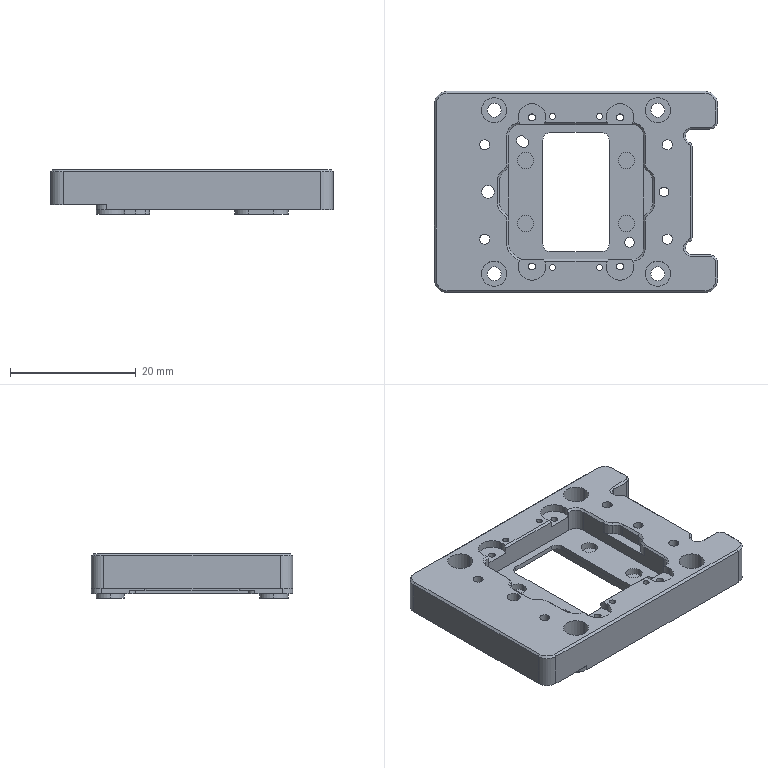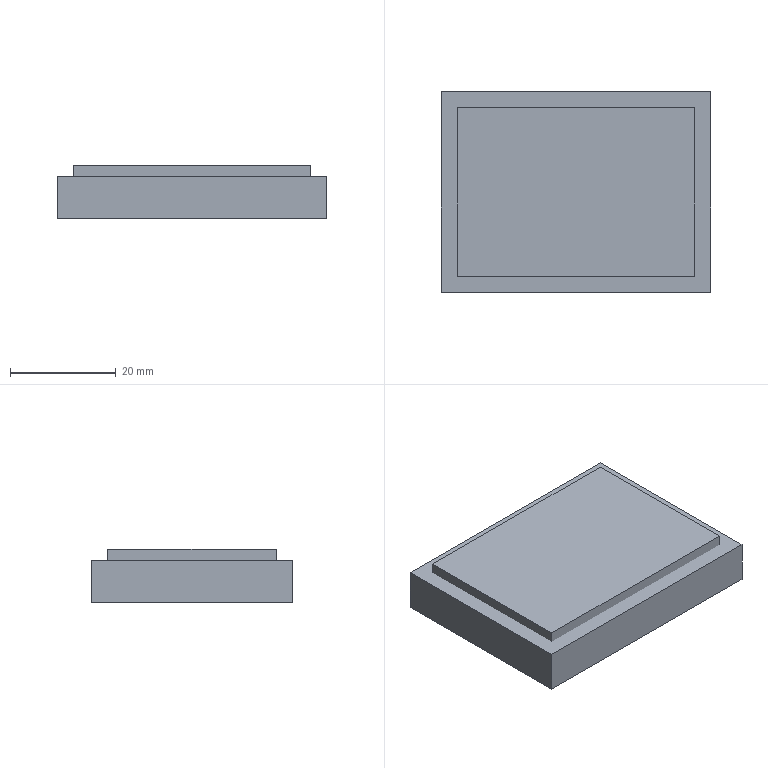CAM job | NX | 3-axis milling, drilling | part box 45 x 32 x 7.05 mm | stock box 51 x 38 x 10.05 mm
Tools:
number,name,description,diameter,corner_radius,flute_length,length,flutes
3,D63,Milling Tool-5 Parameters,63.0,0.0,50.0,75.0,2
1,D6A45,Milling Tool-5 Parameters,6.0,0.0,50.0,75.0,2
11,1.6ZT,Drilling Tool,1.6,0.0,35.0,50.0,2
20,1.55ZT,Drilling Tool,1.55,0.0,35.0,50.0,2
12,2.2ZT,Drilling Tool,2.2,0.0,35.0,50.0,2
13,1.1ZT,Drilling Tool,1.1,0.0,35.0,50.0,2
8,0.95ZT,Drilling Tool,0.95,0.0,35.0,50.0,2
9,2.05ZT,Drilling Tool,2.05,0.0,35.0,50.0,2
6,D6,Milling Tool-5 Parameters,6.0,0.0,50.0,75.0,2
17,D3,Milling Tool-5 Parameters,3.0,0.0,50.0,75.0,2
19,D1.5,Milling Tool-5 Parameters,1.5,0.0,50.0,75.0,2
21,D1,Milling Tool-5 Parameters,1.0,0.0,50.0,75.0,2
18,1.17ZT,Drilling Tool,1.17,0.0,35.0,50.0,2
15,D2,Milling Tool-5 Parameters,2.0,0.0,50.0,75.0,2
15,R0.75,Milling Tool-5 Parameters,0.05,0.025,50.0,75.0,2
Operations:
program,operation,operation_type,tool,method,geometry_group,spindle_rpm,surface_speed,feed_per_tooth,feed_cut,feed_plunge,cut_length_mm,path_length_mm,cut_time_min,machine_time_min
1,FLOOR_WALL,VolumeBased25DMillingOperation,D63,METHOD,A,6500.0,1286.0,0.0962,1250.0,100.0,126.0,180.0,0.1008,0.1062
1,DRILLING,Operation,D6A45,METHOD,A,5000.0,94.0,0.025,250.0,0.0,86.4,459.336,0.3456,0.3829
1,DRILLING_COPY,Operation,1.6ZT,METHOD,A,2000.0,10.0,0.025,100.0,0.0,43.323,215.394,0.4332,0.4504
1,DRILLING_COPY_COPY_1,Operation,1.55ZT,METHOD,A,2000.0,10.0,0.025,100.0,0.0,10.816,81.631,0.1082,0.1152
1,DRILLING_COPY_COPY,Operation,2.2ZT,METHOD,A,1447.0,10.0,0.0346,100.0,0.0,48.844,255.924,0.4884,0.5091
1,DRILLING_COPY_COPY_1_COPY,Operation,1.1ZT,METHOD,A,2000.0,10.0,0.025,100.0,0.0,46.122,213.768,0.4612,0.478
1,DRILLING_COPY_COPY_1_COPY_COPY,Operation,0.95ZT,METHOD,A,2000.0,10.0,0.025,100.0,0.0,37.542,184.425,0.3754,0.3901
1,DRILLING_COPY_COPY_COPY,Operation,2.05ZT,METHOD,A,1447.0,10.0,0.0346,100.0,0.0,10.966,81.932,0.1097,0.1168
1,ADAPTIVE_MILLING,CavityMilling,D6,METHOD,A,9500.0,179.0,0.1579,3000.0,1000.0,3220.322,3711.311,1.462,1.511
1,CAVITY_MILL,CavityMilling,D3,METHOD,A,9500.0,89.0,0.0579,1100.0,100.0,1664.324,5930.193,1.513,1.94
1,HOLE_MILLING,CylinderMilling,D3,METHOD,A,9500.0,89.0,0.0658,1250.0,100.0,239.206,567.206,0.1914,0.2242
1,FLOOR_WALL_1,VolumeBased25DMillingOperation,D3,METHOD,A,9500.0,89.0,0.0526,1000.0,100.0,79.093,512.585,0.0791,0.1224
1,FLOOR_WALL_1_COPY,VolumeBased25DMillingOperation,D3,METHOD,A,9500.0,89.0,0.0526,1000.0,100.0,215.049,280.75,0.215,0.2216
1,ZLEVEL_PROFILE,ZLevelMilling,D3,METHOD,A,9500.0,89.0,0.0526,1000.0,100.0,342.681,413.926,0.3427,0.3498
1,ZLEVEL_PROFILE_COPY,ZLevelMilling,D3,METHOD,A,9500.0,89.0,0.0526,1000.0,100.0,51.989,118.189,0.052,0.0586
1,HOLE_MILLING_COPY,CylinderMilling,D1.5,METHOD,A,9500.0,44.0,0.05,950.0,100.0,235.081,544.081,0.2475,0.2784
1,CAVITY_MILL_COPY,CavityMilling,D1.5,METHOD,A,9500.0,44.0,0.05,950.0,100.0,64.852,395.452,0.0683,0.1013
1,CAVITY_MILL_COPY_COPY,CavityMilling,D1.5,METHOD,A,9500.0,44.0,0.05,950.0,100.0,456.438,779.34,0.4805,0.5128
1,ZLEVEL_PROFILE_1,ZLevelMilling,D1,METHOD,A,9500.0,29.0,0.0447,850.0,100.0,73.019,141.719,0.0859,0.0928
1,PLANAR_MILL,PlanarMilling,D6A45,METHOD,A,9500.0,179.0,0.0658,1250.0,100.0,168.983,227.983,0.1352,0.1411
1,PLANAR_MILL_COPY_1,PlanarMilling,D6A45,METHOD,A,9500.0,179.0,0.0658,1250.0,100.0,83.014,142.014,0.0664,0.0723
1,PLANAR_MILL_COPY_1_COPY,PlanarMilling,D6A45,METHOD,A,9500.0,179.0,0.0658,1250.0,100.0,28.306,165.306,0.0226,0.0363
1,PLANAR_MILL_COPY,PlanarMilling,D6A45,METHOD,A,9500.0,179.0,0.0658,1250.0,100.0,80.89,755.517,0.0647,0.1322
1,PLANAR_MILL_COPY_COPY,PlanarMilling,D6A45,METHOD,A,9500.0,179.0,0.0658,1250.0,100.0,50.331,337.067,0.0403,0.0689
1,刀补3,VolumeBased25DMillingOperation,D3,METHOD,A,9500.0,89.0,0.0526,1000.0,100.0,77.678,143.378,0.0777,0.0842
1,刀补21,ZLevelMilling,D1,METHOD,A,9500.0,29.0,0.0447,850.0,100.0,6.939,74.639,0.0082,0.0149
2,FLOOR_WALL_COPY,VolumeBased25DMillingOperation,D63,METHOD,B,6500.0,1286.0,0.0962,1250.0,100.0,360.0,744.001,0.288,0.3264
2,DRILLING_COPY_1,Operation,D6A45,METHOD,B,5000.0,94.0,0.025,250.0,0.0,7.2,109.158,0.0288,0.039
2,DRILLING_COPY_COPY_1_COPY_COPY_1,Operation,1.17ZT,METHOD,B,2000.0,10.0,0.025,100.0,0.0,12.703,120.164,0.127,0.1378
2,FLOOR_WALL_2,VolumeBased25DMillingOperation,D6,METHOD,B,9500.0,179.0,0.1316,2500.0,1000.0,2722.049,3099.009,1.107,1.145
2,CAVITY_MILL_COPY_1,CavityMilling,D3,METHOD,B,9500.0,89.0,0.0579,1100.0,100.0,21.873,161.567,0.0199,0.0339
2,CAVITY_MILL_COPY_1_COPY,CavityMilling,D3,METHOD,B,9500.0,89.0,0.0579,1100.0,100.0,244.638,584.875,0.2224,0.2564
2,FLOOR_WALL_1_COPY_COPY,VolumeBased25DMillingOperation,D3,METHOD,B,9500.0,89.0,0.0526,1000.0,100.0,1644.763,2949.854,1.645,1.775
2,CAVITY_MILL_COPY_1_COPY_COPY,CavityMilling,D2,METHOD,B,9500.0,59.0,0.0526,1000.0,100.0,341.533,525.734,0.3415,0.36
2,PLANAR_MILL_COPY_COPY_COPY,PlanarMilling,D6A45,METHOD,B,9500.0,179.0,0.0658,1250.0,100.0,136.932,821.732,0.1095,0.178
2,PLANAR_MILL_COPY_COPY_COPY_COPY,PlanarMilling,D6A45,METHOD,B,9500.0,179.0,0.0658,1250.0,100.0,172.209,795.616,0.1378,0.2001
2,PLANAR_MILL_COPY_COPY_COPY_COPY_COPY,PlanarMilling,D6A45,METHOD,B,9500.0,179.0,0.0658,1250.0,100.0,48.989,111.989,0.0392,0.0455
2,PLANAR_MILL_COPY_COPY_COPY_COPY_COPY_COPY,PlanarMilling,D6A45,METHOD,B,9500.0,179.0,0.0658,1250.0,100.0,39.853,193.202,0.0319,0.0472
2,ZLEVEL_PROFILE_2_COPY,ZLevelMilling,R0.75,METHOD,MCS_MILL_COPY_1,9500.0,14.0,0.0658,1250.0,500.0,207.249,1426.727,0.2442,0.3661